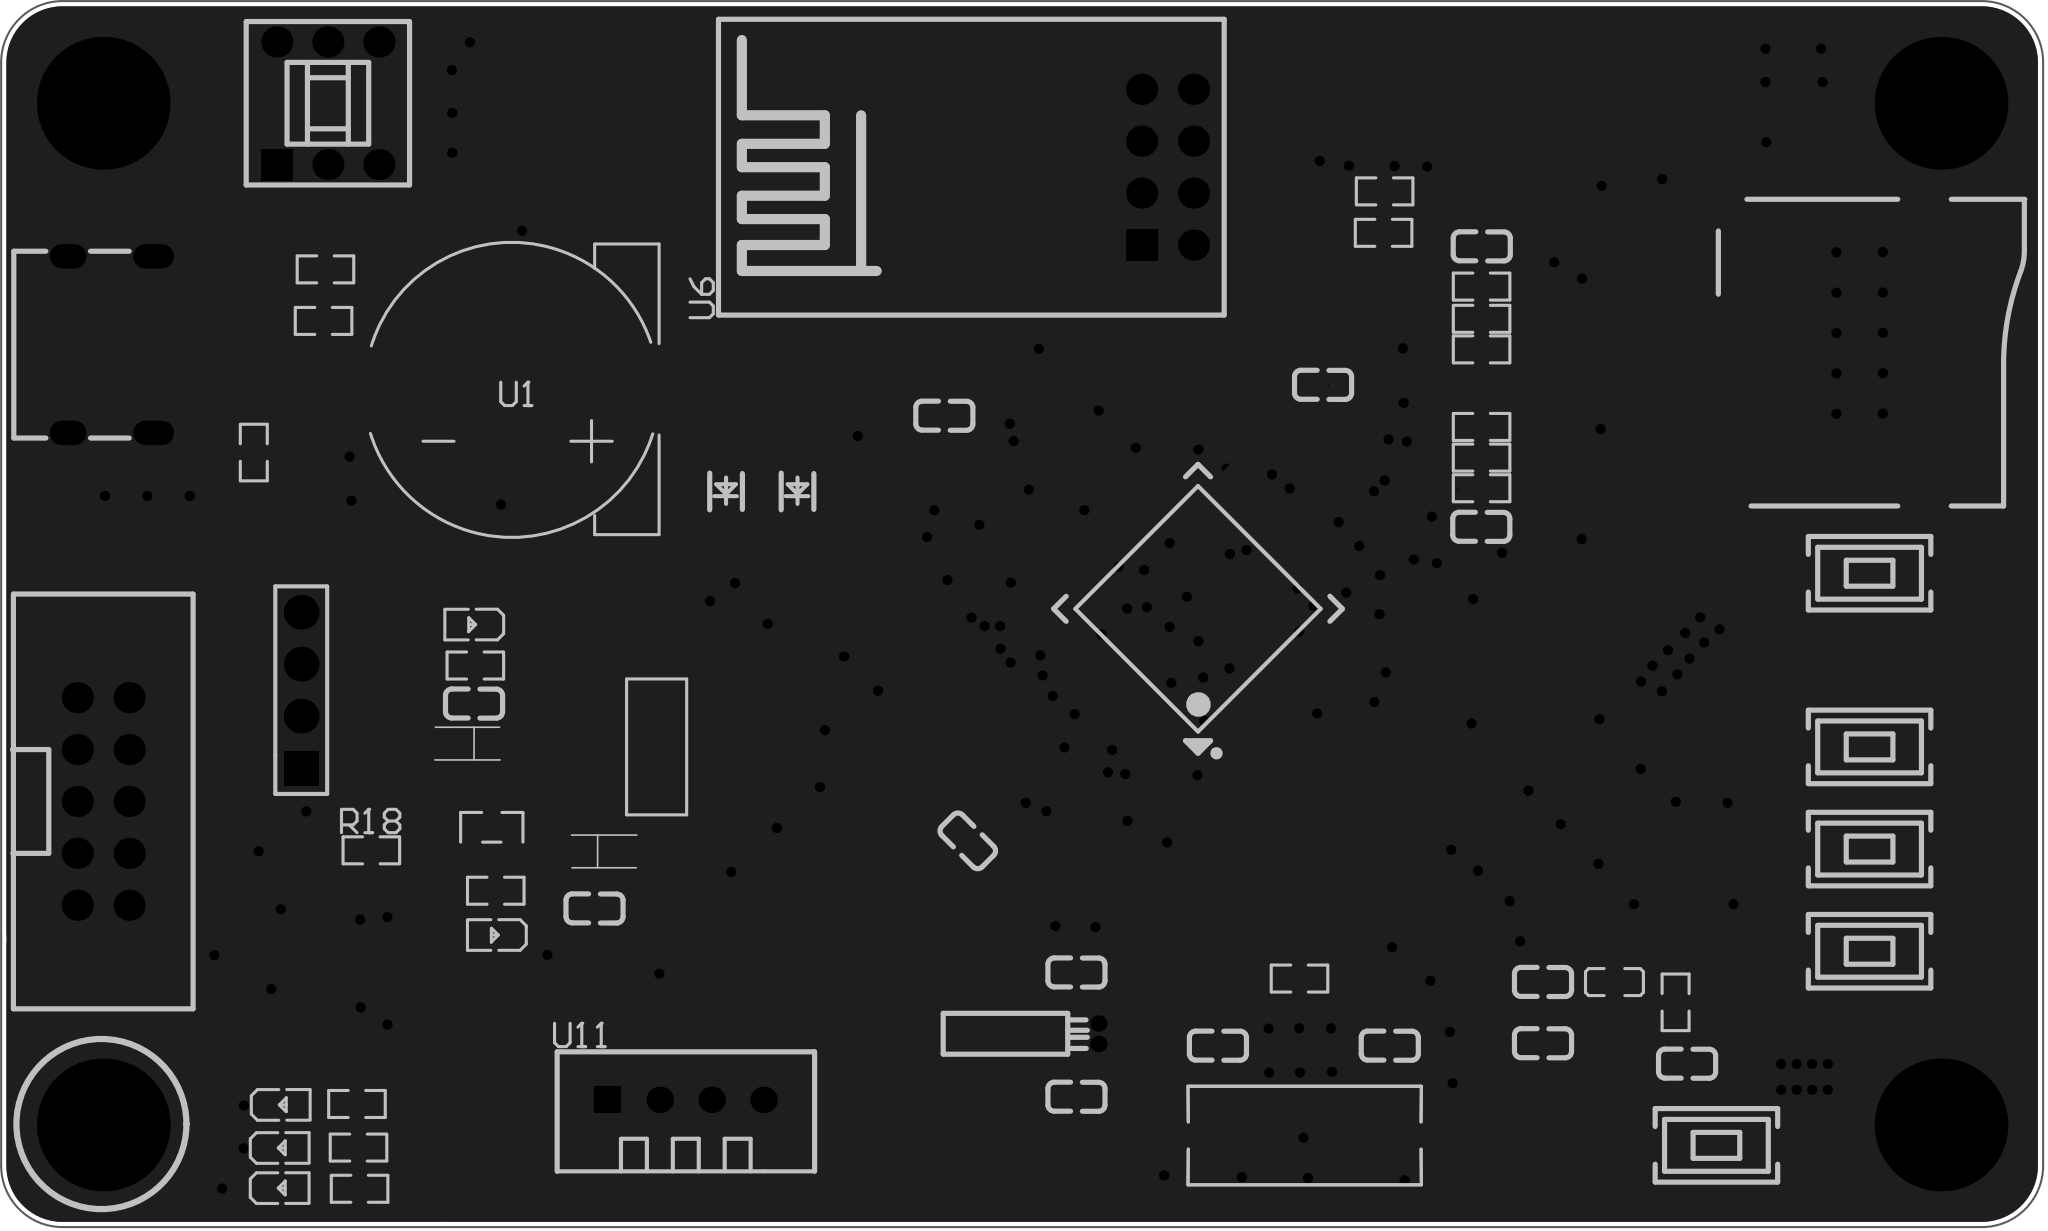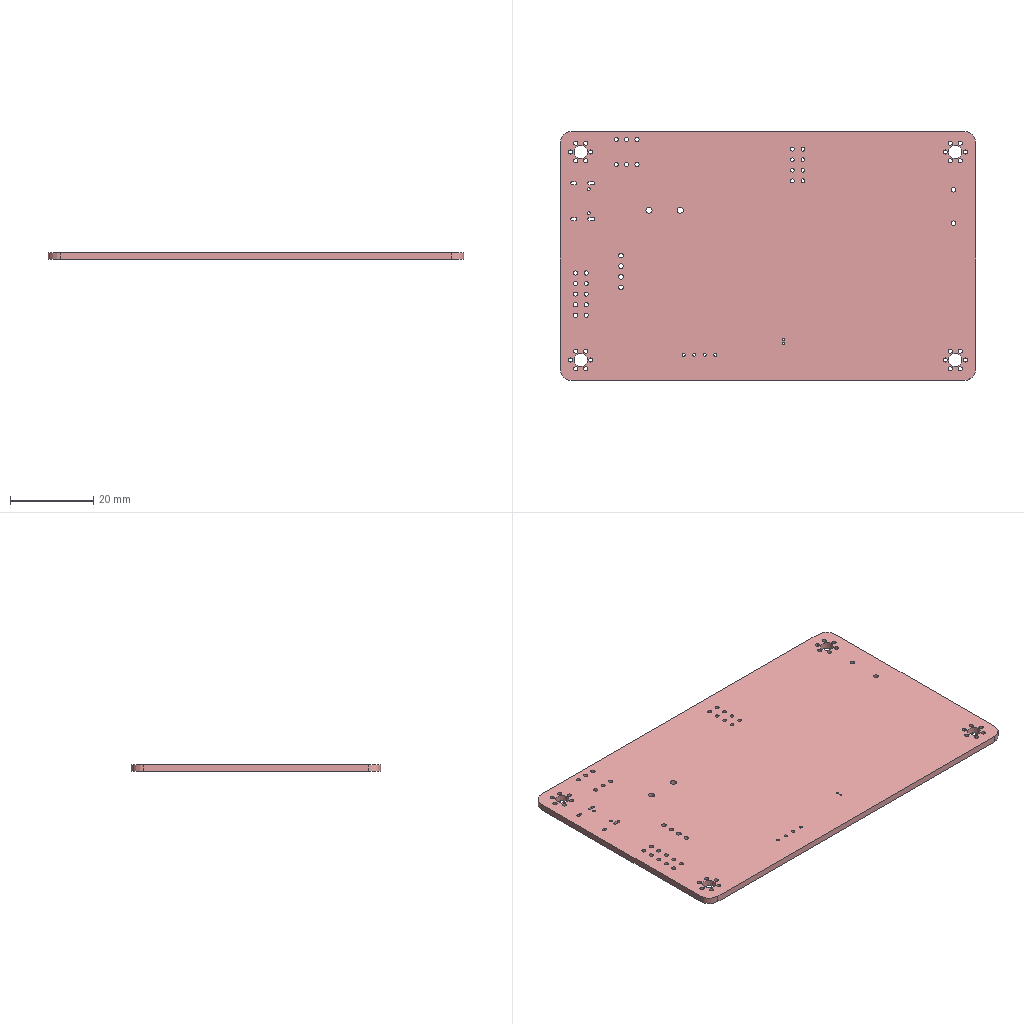Circuit board layout | Altium Designer | box 100 x 60 x 1.6 mm
Layer stack:
# Altium Designer layer stack of  (unit mm; dielectric type: 0 none, 1 core, 2 prepreg, 3 surface material)
index,name,kind,layer,copper_thickness_mm,dielectric_type,dielectric_thickness_mm,dielectric_material,dielectric_constant
0,Top Paste Mask Layer,other,,,,,,
1,Top Silkscreen Layer,other,,,,,,
2,Top Solder Mask Layer,dielectric,,,3,0.01,,3.3
3,Top Layer,copper,Top Layer,0.035,,,,
4,Dielectric1,dielectric,,,3,1.51,FR4,4.5
5,Bottom Layer,copper,Bottom Layer,0.035,,,,
6,Bottom Solder Mask Layer,dielectric,,,3,0.01,,3.3
7,Bottom Silkscreen Layer,other,,,,,,
8,Bottom Paste Mask Layer,other,,,,,,
# drill layer pairs: low layer,high layer
drill_pair,Top Layer,Bottom Layer
Part placement:
Designator,Comment,Layer,Footprint,Center-X(mm),Center-Y(mm),Rotation
U4,STM32F103RCT6,TopLayer,LQFP-64_L10.0-W10.0-P0.50-LS12.0-BL,157.324,110.538,45
X2,32.768kHz,TopLayer,OSC-TH_BD2.0-P0.70-D0.3,152.444,89.74,0
P1,2.54-2*5P box header,TopLayer,IDC-TH_10P-P2.54_C5665,103.711,101.11,270
LED2,LTST-C191KRKT,TopLayer,LED0603-RD,121.829,109.772,180
C8,100pF,TopLayer,C0603,174.211,89.279,180
C3,100nF,TopLayer,C0603,171.203,114.548,0
R5,220Ω,TopLayer,R0603,121.932,107.763,0
C9,100nF,TopLayer,C0603,163.454,121.497,0
U1,CR1220-A,TopLayer,BAT-SMD_CR1220-2,123.711,121.279,180
R3,10kΩ,TopLayer,R0603,166.411,128.939,0
C11,100nF,TopLayer,C0603,146.052,99.174,315
U2,10uF,TopLayer,CASE-A_3216,128.242,98.664,0
U5,10uF,TopLayer,CASE-A_3216,121.547,103.942,180
R2,10kΩ,TopLayer,R0603,166.462,130.967,180
C12,100nF,TopLayer,C0603,144.908,119.986,0
SW3,YTS1C0051AWG00,TopLayer,SW-SMD_L6.1-W3.6-LS8.0,190.211,93.779,0
C4,20pF,TopLayer,C0603,151.378,92.737,0
SW4,YTS1C0051AWG00,TopLayer,SW-SMD_L6.1-W3.6-LS8.0,190.211,98.779,0
SW5,YTS1C0051AWG00,TopLayer,SW-SMD_L6.1-W3.6-LS8.0,190.211,103.779,0
C5,20pF,TopLayer,C0603,151.378,86.656,0
C1,20pF,TopLayer,C0603,158.29,89.161,180
SW6,YTS1C0051AWG00,TopLayer,SW-SMD_L6.1-W3.6-LS8.0,190.211,112.279,0
SW2,YTS1C0051AWG00,TopLayer,SW-SMD_L6.1-W3.6-LS8.0,182.711,84.279,0
C2,20pF,TopLayer,C0603,166.721,89.156,0
R4,1MΩ,TopLayer,R0603,162.294,92.443,180
C7,100pF,TopLayer,C0603,174.211,92.279,180
L1,1uH,TopLayer,L0603,177.711,92.279,180
LED3,LTST-C191KRKT,TopLayer,LED0603-RD,112.4,82.181,0
R14,220,TopLayer,R0603,116.263,82.155,0
USB1,KH-TYPE-C-16P,TopLayer,USB-C-SMD_KH-TYPE-C-16P,104.41,123.467,270
C6,100nF,TopLayer,C0603,127.776,95.871,0
U7,,TopLayer,M3_花孔,103.711,135.279,0
C10,100nF,TopLayer,C0603,121.876,105.897,0
TF1,TF_CARD_SELF,TopLayer,TF-SMD_TF-15-15,187.711,122.939,0
R7,10kΩ,TopLayer,R0603,171.211,126.308,180
U8,,TopLayer,M3_花孔,193.711,135.279,0
R8,10kΩ,TopLayer,R0603,171.211,124.73,180
U9,,TopLayer,M3_花孔,193.711,85.279,0
C13,100nF,TopLayer,C0603,171.211,128.279,180
U10,,TopLayer,M3_花孔,103.711,85.279,0
SW1,XKB8080-Z,TopLayer,SW-TH_6P-L8.0-W8.0-P2.50,114.711,135.279,0
R10,10kΩ,TopLayer,R0603,171.211,119.439,180
R11,10kΩ,TopLayer,R0603,171.211,117.939,180
R18,10K,TopLayer,R0603,116.839,98.718,0
R12,10kΩ,TopLayer,R0603,171.211,116.439,180
R9,10kΩ,TopLayer,R0603,171.211,123.234,180
R13,10kΩ,TopLayer,R0603,180.711,91.279,90
C14,1uF,TopLayer,C0603,181.266,88.279,180
R1,220Ω,TopLayer,R0603,122.932,96.741,0
X1,8MHz,TopLayer,HC-49S_L11.4-W4.8,162.546,84.76,180
U3,AMS1117-3.3,TopLayer,SOT-223-3_L6.5-W3.4-P2.30-LS7.0-BR,130.711,103.779,180
H4,826629-4,TopLayer,HDR-TH_4P-P2.54-V-M-1,113.406,106.557,90
D2,LL4148,TopLayer,LL-34_L3.5-W1.5-RD,137.711,116.279,90
D1,LL4148,TopLayer,LL-34_L3.5-W1.5-RD,134.211,116.279,90
LED1,KT-0603R,TopLayer,LED0603-RD,122.936,94.579,180
Q1,S8050,TopLayer,SOT-23-3_L2.9-W1.3-P1.90-LS2.4-BR,122.738,99.846,270
R15,22Ω,TopLayer,R0603,114.499,124.627,0
R16,22Ω,TopLayer,R0603,114.593,127.15,180
R17,1.5kΩ,TopLayer,R0603,111.082,118.185,270
U6,ESP8266-01S,TopLayer,WIFIM-TH_ESP8266-01S,155.835,132.151,90
U11,DHT11,TopLayer,SENSOR-TH_DHT11,132.239,86.508,0
LED4,LTST-C191KRKT,TopLayer,LED0603-RD,112.452,86.254,0
LED5,LTST-C191KRKT,TopLayer,LED0603-RD,112.401,84.145,0
R6,220,TopLayer,R0603,116.135,86.304,0
R19,220,TopLayer,R0603,116.211,84.171,0
Pad and via stacks:
# Altium Designer via and pad stacks of  (unit mm). Each distinct definition once, with the count of objects using it.
# via: kind,start_layer,end_layer,hole_mm,diameter_mm,mode(0 simple;1 top-mid-bottom;2 full stack),diameter_per_layer,count,example_net
# pad: kind,layer,hole_mm,hole_type(0 round;1 square;2 slot),plating,top_size,top_shape(1 round;2 rect;3 octagon;9 rounded rect),mid_size,bottom_size,mode,footprint,size_per_layer,count,example
pad,Top Layer,0,0,plated,2x0.3,1,2x0.3,2x0.3,0,LQFP-64_L10.0-W10.0-P0.50-LS12.0-BL,,32,U4.64
pad,Top Layer,0,0,plated,0.3x2,1,0.3x2,0.3x2,0,LQFP-64_L10.0-W10.0-P0.50-LS12.0-BL,,32,U4.48
pad,Top Layer,0,0,plated,0.8x0.8,2,0.8x0.8,0.8x0.8,0,LED0603-RD,,10,LED2.2
pad,Top Layer,0,0,plated,0.8x0.9,2,0.8x0.9,0.8x0.9,0,C0603,,28,C8.2
pad,Top Layer,0,0,plated,0.8065x0.864,2,0.8065x0.864,0.8065x0.864,0,R0603,,38,R5.2
pad,Top Layer,0,0,plated,4x2.3,2,4x2.3,4x2.3,0,BAT-SMD_CR1220-2,,1,U1.2
pad,Top Layer,0,0,plated,4.4x2.3,2,4.4x2.3,4.4x2.3,0,BAT-SMD_CR1220-2,,1,U1.1
pad,Top Layer,0,0,plated,1.5x1.359,2,1.5x1.359,1.5x1.359,0,CASE-A_3216,,4,U2.1
pad,Top Layer,0,0,plated,2x1.38,2,2x1.38,2x1.38,0,SW-SMD_L6.1-W3.6-LS8.0,,10,SW3.1
pad,Top Layer,0,0,plated,0.8x0.864,2,0.8x0.864,0.8x0.864,0,L0603,,2,L1.1
pad,Top Layer,0,0,plated,0.3x1.3,2,0.3x1.3,0.3x1.3,0,USB-C-SMD_KH-TYPE-C-16P,,16,USB1.A1
pad,Top Layer,0,0,plated,1.6x0.701,2,1.6x0.701,1.6x0.701,0,TF-SMD_TF-15-15,,9,TF1.1
pad,Top Layer,0,0,plated,1.6x1.8,2,1.6x1.8,1.6x1.8,0,TF-SMD_TF-15-15,,1,TF1.10
pad,Top Layer,0,0,plated,2.4x1.6,2,2.4x1.6,2.4x1.6,0,TF-SMD_TF-15-15,,2,TF1.11
pad,Top Layer,0,0,plated,1.399x1.801,2,1.399x1.801,1.399x1.801,0,TF-SMD_TF-15-15,,1,TF1.13
pad,Top Layer,0,0,plated,5.5x1.3,2,5.5x1.3,5.5x1.3,0,HC-49S_L11.4-W4.8,,2,X1.1
pad,Top Layer,0,0,plated,2.5x1.1,2,2.5x1.1,2.5x1.1,0,SOT-223-3_L6.5-W3.4-P2.30-LS7.0-BR,,3,U3.1
pad,Top Layer,0,0,plated,2.34x3.6,2,2.34x3.6,2.34x3.6,0,SOT-223-3_L6.5-W3.4-P2.30-LS7.0-BR,,1,U3.4
pad,Top Layer,0,0,plated,1.1x1.7,2,1.1x1.7,1.1x1.7,0,LL-34_L3.5-W1.5-RD,,4,D2.2
pad,Top Layer,0,0,plated,1.25x0.7,2,1.25x0.7,1.25x0.7,0,SOT-23-3_L2.9-W1.3-P1.90-LS2.4-BR,,3,Q1.1
pad,Multi-Layer,0.5,0,plated,0.8x0.8,1,0.8x0.8,0.8x0.8,0,OSC-TH_BD2.0-P0.70-D0.3,,2,X2.1
pad,Multi-Layer,1,0,plated,1.524x1.524,1,1.524x1.524,1.524x1.524,0,IDC-TH_10P-P2.54_C5665,,10,P1.1
pad,Multi-Layer,0.7,2,plated,1.2x1.8,1,1.2x1.8,1.2x1.8,0,USB-C-SMD_KH-TYPE-C-16P,,2,USB1.3
pad,Multi-Layer,0.7,2,plated,1.2x2,1,1.2x2,1.2x2,0,USB-C-SMD_KH-TYPE-C-16P,,2,USB1.2
pad,Multi-Layer,3.175,0,plated,6.5x6.5,1,6.5x6.5,6.5x6.5,0,M3_\u00BB\u00A8\u00BF\u00D7,,4,U7.1
pad,Multi-Layer,1.016,2,plated,1.016x1.016,1,1.016x1.016,1.016x1.016,0,M3_\u00BB\u00A8\u00BF\u00D7,,24,U7.1
pad,Multi-Layer,1,0,plated,1.524x1.524,1,1.524x1.524,1.524x1.524,0,SW-TH_6P-L8.0-W8.0-P2.50,,5,SW1.3
pad,Multi-Layer,1,0,plated,1.524x1.524,2,1.524x1.524,1.524x1.524,0,SW-TH_6P-L8.0-W8.0-P2.50,,1,SW1.1
pad,Multi-Layer,1.1,0,plated,1.7x1.7,2,1.7x1.7,1.7x1.7,0,HDR-TH_4P-P2.54-V-M-1,,1,H4.1
pad,Multi-Layer,1.1,0,plated,1.7x1.7,1,1.7x1.7,1.7x1.7,0,HDR-TH_4P-P2.54-V-M-1,,3,H4.2
pad,Multi-Layer,0.9144,0,plated,1.524x1.524,1,1.524x1.524,1.524x1.524,0,WIFIM-TH_ESP8266-01S,,7,U6.8
pad,Multi-Layer,0.9144,0,plated,1.524x1.524,2,1.524x1.524,1.524x1.524,0,WIFIM-TH_ESP8266-01S,,1,U6.1
pad,Multi-Layer,0.7112,0,plated,1.295x1.295,2,1.295x1.295,1.295x1.295,0,SENSOR-TH_DHT11,,1,U11.1
pad,Multi-Layer,0.7112,0,plated,1.295x1.295,1,1.295x1.295,1.295x1.295,0,SENSOR-TH_DHT11,,3,U11.2
via,Top Layer,Bottom Layer,0.2997,0.5,0,,190,GND
Copper pours:
name,layer,net,type(0 solid;1 hatched;2 none)
Top Layer-GND,Top Layer,GND,0
Top Layer-D+,Top Layer,D+,0
Bottom Layer-GND,Bottom Layer,GND,0
Bottom Layer-5VOUT,Bottom Layer,5VOUT,0
Design rules, without the lines most boards share:
# Altium Designer design rules of  (exported by Altium Designer, unit mm)
# columns: name | kind | enabled | priority | scope1 | scope2 | descriptor | typed fields (field=value)
otherClearance | 52 | enabled | 1 | All | All | Hole To Hole Clearance (Gap=11.8mil) (All),(All) | gap=0.2997
solderMaskExpansion | 13 | enabled | 2 | All | All | Solder Mask Expansion (Expansion =2.008mil) (All) | expansion=0.051